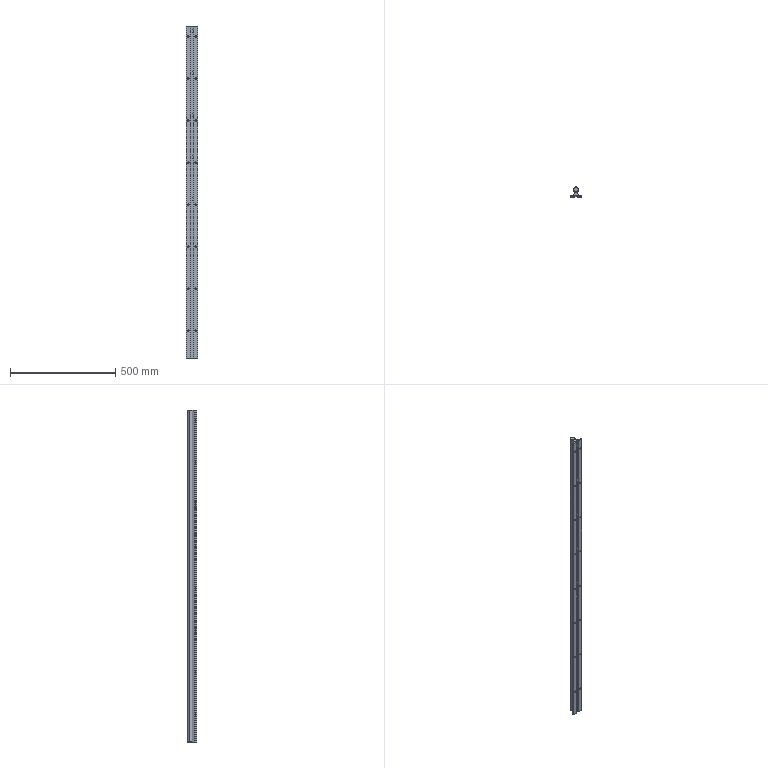Part | SolidWorks | features BaseBody 1 | 1 solid | 97 faces | box 55 x 45.5 x 1580 mm | volume 1553379 mm3 | plane 54 | cylinder 39 | cone 4 | commonest cylinder face diameters 6.6 x32 25 x5 4 x2